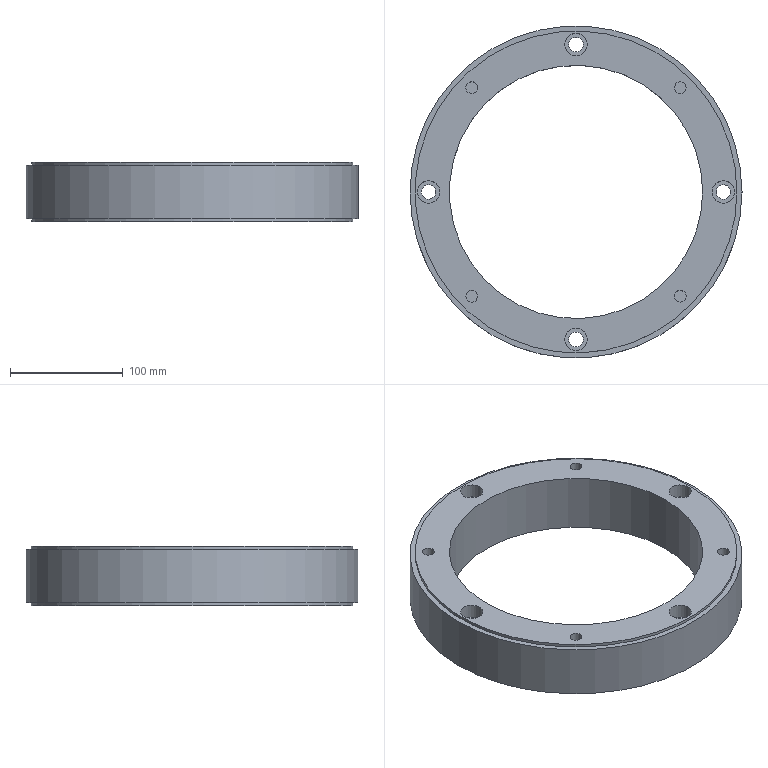Part | NX | 1 solid | 28 faces | box 295 x 295 x 53 mm | volume 1445870 mm3 | cylinder 16 | plane 12 | commonest cylinder face diameters 10.5 x4 13 x4 20 x4 286 x2 225 x1 295 x1
STEP:
#1=CARTESIAN_POINT('',(143.,0.,0.));
#2=VERTEX_POINT('',#1);
#3=CARTESIAN_POINT('',(0.,0.,0.));
#4=DIRECTION('',(0.,0.,1.));
#5=DIRECTION('',(1.,0.,0.));
#6=AXIS2_PLACEMENT_3D('',#3,#4,#5);
#7=CIRCLE('',#6,143.);
#8=EDGE_CURVE('',#2,#2,#7,.T.);
#9=ORIENTED_EDGE('',*,*,#8,.T.);
#10=EDGE_LOOP('',(#9));
#11=FACE_BOUND('',#10,.T.);
#12=CARTESIAN_POINT('',(112.5,0.,0.));
#13=VERTEX_POINT('',#12);
#14=CARTESIAN_POINT('',(0.,0.,0.));
#15=DIRECTION('',(0.,0.,1.));
#16=DIRECTION('',(1.,0.,0.));
#17=AXIS2_PLACEMENT_3D('',#14,#15,#16);
#18=CIRCLE('',#17,112.5);
#19=EDGE_CURVE('',#13,#13,#18,.T.);
#20=ORIENTED_EDGE('',*,*,#19,.F.);
#21=EDGE_LOOP('',(#20));
#22=FACE_BOUND('',#21,.T.);
#23=CARTESIAN_POINT('',(-131.,10.,0.));
#24=VERTEX_POINT('',#23);
#25=CARTESIAN_POINT('',(-131.,0.,0.));
#26=DIRECTION('',(0.,0.,1.));
#27=DIRECTION('',(0.,1.,0.));
#28=AXIS2_PLACEMENT_3D('',#25,#26,#27);
#29=CIRCLE('',#28,10.);
#30=EDGE_CURVE('',#24,#24,#29,.T.);
#31=ORIENTED_EDGE('',*,*,#30,.F.);
#32=EDGE_LOOP('',(#31));
#33=FACE_BOUND('',#32,.T.);
#34=CARTESIAN_POINT('',(-10.,-131.,0.));
#35=VERTEX_POINT('',#34);
#36=CARTESIAN_POINT('',(0.,-131.,0.));
#37=DIRECTION('',(0.,0.,1.));
#38=DIRECTION('',(-1.,0.,0.));
#39=AXIS2_PLACEMENT_3D('',#36,#37,#38);
#40=CIRCLE('',#39,10.);
#41=EDGE_CURVE('',#35,#35,#40,.T.);
#42=ORIENTED_EDGE('',*,*,#41,.F.);
#43=EDGE_LOOP('',(#42));
#44=FACE_BOUND('',#43,.T.);
#45=CARTESIAN_POINT('',(10.,131.,0.));
#46=VERTEX_POINT('',#45);
#47=CARTESIAN_POINT('',(0.,131.,0.));
#48=DIRECTION('',(0.,0.,1.));
#49=DIRECTION('',(1.,0.,0.));
#50=AXIS2_PLACEMENT_3D('',#47,#48,#49);
#51=CIRCLE('',#50,10.);
#52=EDGE_CURVE('',#46,#46,#51,.T.);
#53=ORIENTED_EDGE('',*,*,#52,.F.);
#54=EDGE_LOOP('',(#53));
#55=FACE_BOUND('',#54,.T.);
#56=CARTESIAN_POINT('',(131.,-10.,0.));
#57=VERTEX_POINT('',#56);
#58=CARTESIAN_POINT('',(131.,0.,0.));
#59=DIRECTION('',(0.,0.,1.));
#60=DIRECTION('',(0.,-1.,0.));
#61=AXIS2_PLACEMENT_3D('',#58,#59,#60);
#62=CIRCLE('',#61,10.);
#63=EDGE_CURVE('',#57,#57,#62,.T.);
#64=ORIENTED_EDGE('',*,*,#63,.F.);
#65=EDGE_LOOP('',(#64));
#66=FACE_BOUND('',#65,.T.);
#67=CARTESIAN_POINT('',(97.881,92.631,0.));
#68=VERTEX_POINT('',#67);
#69=CARTESIAN_POINT('',(92.631,92.631,0.));
#70=DIRECTION('',(0.,0.,1.));
#71=DIRECTION('',(1.,0.,0.));
#72=AXIS2_PLACEMENT_3D('',#69,#70,#71);
#73=CIRCLE('',#72,5.25);
#74=EDGE_CURVE('',#68,#68,#73,.T.);
#75=ORIENTED_EDGE('',*,*,#74,.F.);
#76=EDGE_LOOP('',(#75));
#77=FACE_BOUND('',#76,.T.);
#78=CARTESIAN_POINT('',(92.631,-97.881,0.));
#79=VERTEX_POINT('',#78);
#80=CARTESIAN_POINT('',(92.631,-92.631,0.));
#81=DIRECTION('',(0.,0.,1.));
#82=DIRECTION('',(0.,-1.,0.));
#83=AXIS2_PLACEMENT_3D('',#80,#81,#82);
#84=CIRCLE('',#83,5.25);
#85=EDGE_CURVE('',#79,#79,#84,.T.);
#86=ORIENTED_EDGE('',*,*,#85,.F.);
#87=EDGE_LOOP('',(#86));
#88=FACE_BOUND('',#87,.T.);
#89=CARTESIAN_POINT('',(-97.881,-92.631,0.));
#90=VERTEX_POINT('',#89);
#91=CARTESIAN_POINT('',(-92.631,-92.631,0.));
#92=DIRECTION('',(0.,0.,1.));
#93=DIRECTION('',(-1.,0.,0.));
#94=AXIS2_PLACEMENT_3D('',#91,#92,#93);
#95=CIRCLE('',#94,5.25);
#96=EDGE_CURVE('',#90,#90,#95,.T.);
#97=ORIENTED_EDGE('',*,*,#96,.F.);
#98=EDGE_LOOP('',(#97));
#99=FACE_BOUND('',#98,.T.);
#100=CARTESIAN_POINT('',(-92.631,97.881,0.));
#101=VERTEX_POINT('',#100);
#102=CARTESIAN_POINT('',(-92.631,92.631,0.));
#103=DIRECTION('',(0.,0.,-1.));
#104=DIRECTION('',(0.,1.,0.));
#105=AXIS2_PLACEMENT_3D('',#102,#103,#104);
#106=CIRCLE('',#105,5.25);
#107=EDGE_CURVE('',#101,#101,#106,.T.);
#108=ORIENTED_EDGE('',*,*,#107,.T.);
#109=EDGE_LOOP('',(#108));
#110=FACE_BOUND('',#109,.T.);
#111=CARTESIAN_POINT('',(65.5,0.,0.));
#112=DIRECTION('',(0.,0.,1.));
#113=DIRECTION('',(1.,0.,0.));
#114=AXIS2_PLACEMENT_3D('',#111,#112,#113);
#115=PLANE('',#114);
#116=ADVANCED_FACE('',(#11,#22,#33,#44,#55,#66,#77,#88,#99,#110),#115,.T.);
#117=CARTESIAN_POINT('',(-6.5,-131.,-53.));
#118=VERTEX_POINT('',#117);
#119=CARTESIAN_POINT('',(0.,-131.,-53.));
#120=DIRECTION('',(0.,0.,1.));
#121=DIRECTION('',(-1.,0.,0.));
#122=AXIS2_PLACEMENT_3D('',#119,#120,#121);
#123=CIRCLE('',#122,6.5);
#124=EDGE_CURVE('',#118,#118,#123,.T.);
#125=ORIENTED_EDGE('',*,*,#124,.F.);
#126=EDGE_LOOP('',(#125));
#127=FACE_BOUND('',#126,.T.);
#128=CARTESIAN_POINT('',(6.5,-131.,-13.));
#129=VERTEX_POINT('',#128);
#130=CARTESIAN_POINT('',(0.,-131.,-13.));
#131=DIRECTION('',(0.,0.,1.));
#132=DIRECTION('',(1.,0.,0.));
#133=AXIS2_PLACEMENT_3D('',#130,#131,#132);
#134=CIRCLE('',#133,6.5);
#135=EDGE_CURVE('',#129,#129,#134,.F.);
#136=ORIENTED_EDGE('',*,*,#135,.F.);
#137=EDGE_LOOP('',(#136));
#138=FACE_BOUND('',#137,.T.);
#139=CARTESIAN_POINT('',(0.,-131.,-53.));
#140=DIRECTION('',(0.,0.,1.));
#141=DIRECTION('',(1.,0.,0.));
#142=AXIS2_PLACEMENT_3D('',#139,#140,#141);
#143=CYLINDRICAL_SURFACE('',#142,6.5);
#144=ADVANCED_FACE('',(#127,#138),#143,.F.);
#145=CARTESIAN_POINT('',(6.5,131.,-53.));
#146=VERTEX_POINT('',#145);
#147=CARTESIAN_POINT('',(0.,131.,-53.));
#148=DIRECTION('',(0.,0.,1.));
#149=DIRECTION('',(1.,0.,0.));
#150=AXIS2_PLACEMENT_3D('',#147,#148,#149);
#151=CIRCLE('',#150,6.5);
#152=EDGE_CURVE('',#146,#146,#151,.T.);
#153=ORIENTED_EDGE('',*,*,#152,.F.);
#154=EDGE_LOOP('',(#153));
#155=FACE_BOUND('',#154,.T.);
#156=CARTESIAN_POINT('',(6.5,131.,-13.));
#157=VERTEX_POINT('',#156);
#158=CARTESIAN_POINT('',(0.,131.,-13.));
#159=DIRECTION('',(0.,0.,1.));
#160=DIRECTION('',(1.,0.,0.));
#161=AXIS2_PLACEMENT_3D('',#158,#159,#160);
#162=CIRCLE('',#161,6.5);
#163=EDGE_CURVE('',#157,#157,#162,.F.);
#164=ORIENTED_EDGE('',*,*,#163,.F.);
#165=EDGE_LOOP('',(#164));
#166=FACE_BOUND('',#165,.T.);
#167=CARTESIAN_POINT('',(0.,131.,-53.));
#168=DIRECTION('',(0.,0.,1.));
#169=DIRECTION('',(1.,0.,0.));
#170=AXIS2_PLACEMENT_3D('',#167,#168,#169);
#171=CYLINDRICAL_SURFACE('',#170,6.5);
#172=ADVANCED_FACE('',(#155,#166),#171,.F.);
#173=CARTESIAN_POINT('',(131.,-6.5,-53.));
#174=VERTEX_POINT('',#173);
#175=CARTESIAN_POINT('',(131.,0.,-53.));
#176=DIRECTION('',(0.,0.,1.));
#177=DIRECTION('',(0.,-1.,0.));
#178=AXIS2_PLACEMENT_3D('',#175,#176,#177);
#179=CIRCLE('',#178,6.5);
#180=EDGE_CURVE('',#174,#174,#179,.T.);
#181=ORIENTED_EDGE('',*,*,#180,.F.);
#182=EDGE_LOOP('',(#181));
#183=FACE_BOUND('',#182,.T.);
#184=CARTESIAN_POINT('',(137.5,0.,-13.));
#185=VERTEX_POINT('',#184);
#186=CARTESIAN_POINT('',(131.,0.,-13.));
#187=DIRECTION('',(0.,0.,1.));
#188=DIRECTION('',(1.,0.,0.));
#189=AXIS2_PLACEMENT_3D('',#186,#187,#188);
#190=CIRCLE('',#189,6.5);
#191=EDGE_CURVE('',#185,#185,#190,.F.);
#192=ORIENTED_EDGE('',*,*,#191,.F.);
#193=EDGE_LOOP('',(#192));
#194=FACE_BOUND('',#193,.T.);
#195=CARTESIAN_POINT('',(131.,0.,-53.));
#196=DIRECTION('',(0.,0.,1.));
#197=DIRECTION('',(1.,0.,0.));
#198=AXIS2_PLACEMENT_3D('',#195,#196,#197);
#199=CYLINDRICAL_SURFACE('',#198,6.5);
#200=ADVANCED_FACE('',(#183,#194),#199,.F.);
#201=CARTESIAN_POINT('',(-131.,6.5,-53.));
#202=VERTEX_POINT('',#201);
#203=CARTESIAN_POINT('',(-131.,0.,-53.));
#204=DIRECTION('',(0.,0.,1.));
#205=DIRECTION('',(0.,1.,0.));
#206=AXIS2_PLACEMENT_3D('',#203,#204,#205);
#207=CIRCLE('',#206,6.5);
#208=EDGE_CURVE('',#202,#202,#207,.T.);
#209=ORIENTED_EDGE('',*,*,#208,.F.);
#210=EDGE_LOOP('',(#209));
#211=FACE_BOUND('',#210,.T.);
#212=CARTESIAN_POINT('',(-124.5,0.,-13.));
#213=VERTEX_POINT('',#212);
#214=CARTESIAN_POINT('',(-131.,0.,-13.));
#215=DIRECTION('',(0.,0.,1.));
#216=DIRECTION('',(1.,0.,0.));
#217=AXIS2_PLACEMENT_3D('',#214,#215,#216);
#218=CIRCLE('',#217,6.5);
#219=EDGE_CURVE('',#213,#213,#218,.F.);
#220=ORIENTED_EDGE('',*,*,#219,.F.);
#221=EDGE_LOOP('',(#220));
#222=FACE_BOUND('',#221,.T.);
#223=CARTESIAN_POINT('',(-131.,0.,-53.));
#224=DIRECTION('',(0.,0.,1.));
#225=DIRECTION('',(1.,0.,0.));
#226=AXIS2_PLACEMENT_3D('',#223,#224,#225);
#227=CYLINDRICAL_SURFACE('',#226,6.5);
#228=ADVANCED_FACE('',(#211,#222),#227,.F.);
#229=CARTESIAN_POINT('',(147.5,0.,-2.6));
#230=VERTEX_POINT('',#229);
#231=CARTESIAN_POINT('',(0.,0.,-2.6));
#232=DIRECTION('',(0.,0.,-1.));
#233=DIRECTION('',(1.,0.,0.));
#234=AXIS2_PLACEMENT_3D('',#231,#232,#233);
#235=CIRCLE('',#234,147.5);
#236=EDGE_CURVE('',#230,#230,#235,.T.);
#237=ORIENTED_EDGE('',*,*,#236,.T.);
#238=EDGE_LOOP('',(#237));
#239=FACE_BOUND('',#238,.T.);
#240=CARTESIAN_POINT('',(147.5,0.,-50.4));
#241=VERTEX_POINT('',#240);
#242=CARTESIAN_POINT('',(0.,0.,-50.4));
#243=DIRECTION('',(0.,0.,-1.));
#244=DIRECTION('',(1.,0.,0.));
#245=AXIS2_PLACEMENT_3D('',#242,#243,#244);
#246=CIRCLE('',#245,147.5);
#247=EDGE_CURVE('',#241,#241,#246,.T.);
#248=ORIENTED_EDGE('',*,*,#247,.F.);
#249=EDGE_LOOP('',(#248));
#250=FACE_BOUND('',#249,.T.);
#251=CARTESIAN_POINT('',(0.,0.,-53.));
#252=DIRECTION('',(0.,0.,1.));
#253=DIRECTION('',(1.,0.,0.));
#254=AXIS2_PLACEMENT_3D('',#251,#252,#253);
#255=CYLINDRICAL_SURFACE('',#254,147.5);
#256=ADVANCED_FACE('',(#239,#250),#255,.T.);
#257=ORIENTED_EDGE('',*,*,#208,.T.);
#258=EDGE_LOOP('',(#257));
#259=FACE_BOUND('',#258,.T.);
#260=CARTESIAN_POINT('',(112.5,0.,-53.));
#261=VERTEX_POINT('',#260);
#262=CARTESIAN_POINT('',(0.,0.,-53.));
#263=DIRECTION('',(0.,0.,1.));
#264=DIRECTION('',(1.,0.,0.));
#265=AXIS2_PLACEMENT_3D('',#262,#263,#264);
#266=CIRCLE('',#265,112.5);
#267=EDGE_CURVE('',#261,#261,#266,.T.);
#268=ORIENTED_EDGE('',*,*,#267,.T.);
#269=EDGE_LOOP('',(#268));
#270=FACE_BOUND('',#269,.T.);
#271=ORIENTED_EDGE('',*,*,#124,.T.);
#272=EDGE_LOOP('',(#271));
#273=FACE_BOUND('',#272,.T.);
#274=ORIENTED_EDGE('',*,*,#152,.T.);
#275=EDGE_LOOP('',(#274));
#276=FACE_BOUND('',#275,.T.);
#277=ORIENTED_EDGE('',*,*,#180,.T.);
#278=EDGE_LOOP('',(#277));
#279=FACE_BOUND('',#278,.T.);
#280=CARTESIAN_POINT('',(143.,0.,-53.));
#281=VERTEX_POINT('',#280);
#282=CARTESIAN_POINT('',(0.,0.,-53.));
#283=DIRECTION('',(0.,0.,1.));
#284=DIRECTION('',(1.,0.,0.));
#285=AXIS2_PLACEMENT_3D('',#282,#283,#284);
#286=CIRCLE('',#285,143.);
#287=EDGE_CURVE('',#281,#281,#286,.T.);
#288=ORIENTED_EDGE('',*,*,#287,.F.);
#289=EDGE_LOOP('',(#288));
#290=FACE_BOUND('',#289,.T.);
#291=CARTESIAN_POINT('',(65.5,0.,-53.));
#292=DIRECTION('',(0.,0.,1.));
#293=DIRECTION('',(1.,0.,0.));
#294=AXIS2_PLACEMENT_3D('',#291,#292,#293);
#295=PLANE('',#294);
#296=ADVANCED_FACE('',(#259,#270,#273,#276,#279,#290),#295,.F.);
#297=ORIENTED_EDGE('',*,*,#267,.F.);
#298=EDGE_LOOP('',(#297));
#299=FACE_BOUND('',#298,.T.);
#300=ORIENTED_EDGE('',*,*,#19,.T.);
#301=EDGE_LOOP('',(#300));
#302=FACE_BOUND('',#301,.T.);
#303=CARTESIAN_POINT('',(0.,0.,-53.));
#304=DIRECTION('',(0.,0.,1.));
#305=DIRECTION('',(1.,0.,0.));
#306=AXIS2_PLACEMENT_3D('',#303,#304,#305);
#307=CYLINDRICAL_SURFACE('',#306,112.5);
#308=ADVANCED_FACE('',(#299,#302),#307,.F.);
#309=CARTESIAN_POINT('',(143.,0.,-2.6));
#310=VERTEX_POINT('',#309);
#311=CARTESIAN_POINT('',(0.,0.,-2.6));
#312=DIRECTION('',(0.,0.,1.));
#313=DIRECTION('',(1.,0.,0.));
#314=AXIS2_PLACEMENT_3D('',#311,#312,#313);
#315=CIRCLE('',#314,143.);
#316=EDGE_CURVE('',#310,#310,#315,.F.);
#317=ORIENTED_EDGE('',*,*,#316,.F.);
#318=EDGE_LOOP('',(#317));
#319=FACE_BOUND('',#318,.T.);
#320=ORIENTED_EDGE('',*,*,#8,.F.);
#321=EDGE_LOOP('',(#320));
#322=FACE_BOUND('',#321,.T.);
#323=CARTESIAN_POINT('',(0.,0.,-2.6));
#324=DIRECTION('',(0.,0.,1.));
#325=DIRECTION('',(1.,0.,0.));
#326=AXIS2_PLACEMENT_3D('',#323,#324,#325);
#327=CYLINDRICAL_SURFACE('',#326,143.);
#328=ADVANCED_FACE('',(#319,#322),#327,.T.);
#329=ORIENTED_EDGE('',*,*,#236,.F.);
#330=EDGE_LOOP('',(#329));
#331=FACE_BOUND('',#330,.T.);
#332=ORIENTED_EDGE('',*,*,#316,.T.);
#333=EDGE_LOOP('',(#332));
#334=FACE_BOUND('',#333,.T.);
#335=CARTESIAN_POINT('',(0.,0.,-2.6));
#336=DIRECTION('',(0.,0.,-1.));
#337=DIRECTION('',(-1.,0.,0.));
#338=AXIS2_PLACEMENT_3D('',#335,#336,#337);
#339=PLANE('',#338);
#340=ADVANCED_FACE('',(#331,#334),#339,.F.);
#341=CARTESIAN_POINT('',(143.,0.,-50.4));
#342=VERTEX_POINT('',#341);
#343=CARTESIAN_POINT('',(0.,0.,-50.4));
#344=DIRECTION('',(0.,0.,1.));
#345=DIRECTION('',(1.,0.,0.));
#346=AXIS2_PLACEMENT_3D('',#343,#344,#345);
#347=CIRCLE('',#346,143.);
#348=EDGE_CURVE('',#342,#342,#347,.F.);
#349=ORIENTED_EDGE('',*,*,#348,.T.);
#350=EDGE_LOOP('',(#349));
#351=FACE_BOUND('',#350,.T.);
#352=ORIENTED_EDGE('',*,*,#287,.T.);
#353=EDGE_LOOP('',(#352));
#354=FACE_BOUND('',#353,.T.);
#355=CARTESIAN_POINT('',(0.,0.,-50.4));
#356=DIRECTION('',(0.,0.,-1.));
#357=DIRECTION('',(-1.,0.,0.));
#358=AXIS2_PLACEMENT_3D('',#355,#356,#357);
#359=CYLINDRICAL_SURFACE('',#358,143.);
#360=ADVANCED_FACE('',(#351,#354),#359,.T.);
#361=ORIENTED_EDGE('',*,*,#247,.T.);
#362=EDGE_LOOP('',(#361));
#363=FACE_BOUND('',#362,.T.);
#364=ORIENTED_EDGE('',*,*,#348,.F.);
#365=EDGE_LOOP('',(#364));
#366=FACE_BOUND('',#365,.T.);
#367=CARTESIAN_POINT('',(0.,0.,-50.4));
#368=DIRECTION('',(0.,0.,-1.));
#369=DIRECTION('',(-1.,0.,0.));
#370=AXIS2_PLACEMENT_3D('',#367,#368,#369);
#371=PLANE('',#370);
#372=ADVANCED_FACE('',(#363,#366),#371,.T.);
#373=CARTESIAN_POINT('',(-131.,10.,-13.));
#374=VERTEX_POINT('',#373);
#375=CARTESIAN_POINT('',(-131.,0.,-13.));
#376=DIRECTION('',(0.,0.,1.));
#377=DIRECTION('',(0.,1.,0.));
#378=AXIS2_PLACEMENT_3D('',#375,#376,#377);
#379=CIRCLE('',#378,10.);
#380=EDGE_CURVE('',#374,#374,#379,.F.);
#381=ORIENTED_EDGE('',*,*,#380,.F.);
#382=EDGE_LOOP('',(#381));
#383=FACE_BOUND('',#382,.T.);
#384=ORIENTED_EDGE('',*,*,#219,.T.);
#385=EDGE_LOOP('',(#384));
#386=FACE_BOUND('',#385,.T.);
#387=CARTESIAN_POINT('',(-131.,0.,-13.));
#388=DIRECTION('',(0.,0.,1.));
#389=DIRECTION('',(1.,0.,0.));
#390=AXIS2_PLACEMENT_3D('',#387,#388,#389);
#391=PLANE('',#390);
#392=ADVANCED_FACE('',(#383,#386),#391,.T.);
#393=ORIENTED_EDGE('',*,*,#380,.T.);
#394=EDGE_LOOP('',(#393));
#395=FACE_BOUND('',#394,.T.);
#396=ORIENTED_EDGE('',*,*,#30,.T.);
#397=EDGE_LOOP('',(#396));
#398=FACE_BOUND('',#397,.T.);
#399=CARTESIAN_POINT('',(-131.,0.,-13.));
#400=DIRECTION('',(0.,0.,1.));
#401=DIRECTION('',(1.,0.,0.));
#402=AXIS2_PLACEMENT_3D('',#399,#400,#401);
#403=CYLINDRICAL_SURFACE('',#402,10.);
#404=ADVANCED_FACE('',(#395,#398),#403,.F.);
#405=CARTESIAN_POINT('',(131.,-10.,-13.));
#406=VERTEX_POINT('',#405);
#407=CARTESIAN_POINT('',(131.,0.,-13.));
#408=DIRECTION('',(0.,0.,1.));
#409=DIRECTION('',(0.,-1.,0.));
#410=AXIS2_PLACEMENT_3D('',#407,#408,#409);
#411=CIRCLE('',#410,10.);
#412=EDGE_CURVE('',#406,#406,#411,.F.);
#413=ORIENTED_EDGE('',*,*,#412,.F.);
#414=EDGE_LOOP('',(#413));
#415=FACE_BOUND('',#414,.T.);
#416=ORIENTED_EDGE('',*,*,#191,.T.);
#417=EDGE_LOOP('',(#416));
#418=FACE_BOUND('',#417,.T.);
#419=CARTESIAN_POINT('',(131.,0.,-13.));
#420=DIRECTION('',(0.,0.,1.));
#421=DIRECTION('',(1.,0.,0.));
#422=AXIS2_PLACEMENT_3D('',#419,#420,#421);
#423=PLANE('',#422);
#424=ADVANCED_FACE('',(#415,#418),#423,.T.);
#425=ORIENTED_EDGE('',*,*,#412,.T.);
#426=EDGE_LOOP('',(#425));
#427=FACE_BOUND('',#426,.T.);
#428=ORIENTED_EDGE('',*,*,#63,.T.);
#429=EDGE_LOOP('',(#428));
#430=FACE_BOUND('',#429,.T.);
#431=CARTESIAN_POINT('',(131.,0.,-13.));
#432=DIRECTION('',(0.,0.,1.));
#433=DIRECTION('',(1.,0.,0.));
#434=AXIS2_PLACEMENT_3D('',#431,#432,#433);
#435=CYLINDRICAL_SURFACE('',#434,10.);
#436=ADVANCED_FACE('',(#427,#430),#435,.F.);
#437=CARTESIAN_POINT('',(10.,131.,-13.));
#438=VERTEX_POINT('',#437);
#439=CARTESIAN_POINT('',(0.,131.,-13.));
#440=DIRECTION('',(0.,0.,1.));
#441=DIRECTION('',(1.,0.,0.));
#442=AXIS2_PLACEMENT_3D('',#439,#440,#441);
#443=CIRCLE('',#442,10.);
#444=EDGE_CURVE('',#438,#438,#443,.F.);
#445=ORIENTED_EDGE('',*,*,#444,.F.);
#446=EDGE_LOOP('',(#445));
#447=FACE_BOUND('',#446,.T.);
#448=ORIENTED_EDGE('',*,*,#163,.T.);
#449=EDGE_LOOP('',(#448));
#450=FACE_BOUND('',#449,.T.);
#451=CARTESIAN_POINT('',(0.,131.,-13.));
#452=DIRECTION('',(0.,0.,1.));
#453=DIRECTION('',(1.,0.,0.));
#454=AXIS2_PLACEMENT_3D('',#451,#452,#453);
#455=PLANE('',#454);
#456=ADVANCED_FACE('',(#447,#450),#455,.T.);
#457=ORIENTED_EDGE('',*,*,#444,.T.);
#458=EDGE_LOOP('',(#457));
#459=FACE_BOUND('',#458,.T.);
#460=ORIENTED_EDGE('',*,*,#52,.T.);
#461=EDGE_LOOP('',(#460));
#462=FACE_BOUND('',#461,.T.);
#463=CARTESIAN_POINT('',(0.,131.,-13.));
#464=DIRECTION('',(0.,0.,1.));
#465=DIRECTION('',(1.,0.,0.));
#466=AXIS2_PLACEMENT_3D('',#463,#464,#465);
#467=CYLINDRICAL_SURFACE('',#466,10.);
#468=ADVANCED_FACE('',(#459,#462),#467,.F.);
#469=CARTESIAN_POINT('',(-10.,-131.,-13.));
#470=VERTEX_POINT('',#469);
#471=CARTESIAN_POINT('',(0.,-131.,-13.));
#472=DIRECTION('',(0.,0.,1.));
#473=DIRECTION('',(-1.,0.,0.));
#474=AXIS2_PLACEMENT_3D('',#471,#472,#473);
#475=CIRCLE('',#474,10.);
#476=EDGE_CURVE('',#470,#470,#475,.F.);
#477=ORIENTED_EDGE('',*,*,#476,.F.);
#478=EDGE_LOOP('',(#477));
#479=FACE_BOUND('',#478,.T.);
#480=ORIENTED_EDGE('',*,*,#135,.T.);
#481=EDGE_LOOP('',(#480));
#482=FACE_BOUND('',#481,.T.);
#483=CARTESIAN_POINT('',(0.,-131.,-13.));
#484=DIRECTION('',(0.,0.,1.));
#485=DIRECTION('',(1.,0.,0.));
#486=AXIS2_PLACEMENT_3D('',#483,#484,#485);
#487=PLANE('',#486);
#488=ADVANCED_FACE('',(#479,#482),#487,.T.);
#489=ORIENTED_EDGE('',*,*,#476,.T.);
#490=EDGE_LOOP('',(#489));
#491=FACE_BOUND('',#490,.T.);
#492=ORIENTED_EDGE('',*,*,#41,.T.);
#493=EDGE_LOOP('',(#492));
#494=FACE_BOUND('',#493,.T.);
#495=CARTESIAN_POINT('',(0.,-131.,-13.));
#496=DIRECTION('',(0.,0.,1.));
#497=DIRECTION('',(1.,0.,0.));
#498=AXIS2_PLACEMENT_3D('',#495,#496,#497);
#499=CYLINDRICAL_SURFACE('',#498,10.);
#500=ADVANCED_FACE('',(#491,#494),#499,.F.);
#501=CARTESIAN_POINT('',(97.881,92.631,-30.));
#502=VERTEX_POINT('',#501);
#503=CARTESIAN_POINT('',(92.631,92.631,-30.));
#504=DIRECTION('',(0.,0.,1.));
#505=DIRECTION('',(1.,0.,0.));
#506=AXIS2_PLACEMENT_3D('',#503,#504,#505);
#507=CIRCLE('',#506,5.25);
#508=EDGE_CURVE('',#502,#502,#507,.F.);
#509=ORIENTED_EDGE('',*,*,#508,.T.);
#510=EDGE_LOOP('',(#509));
#511=FACE_BOUND('',#510,.T.);
#512=ORIENTED_EDGE('',*,*,#74,.T.);
#513=EDGE_LOOP('',(#512));
#514=FACE_BOUND('',#513,.T.);
#515=CARTESIAN_POINT('',(92.631,92.631,-30.));
#516=DIRECTION('',(0.,0.,1.));
#517=DIRECTION('',(1.,0.,0.));
#518=AXIS2_PLACEMENT_3D('',#515,#516,#517);
#519=CYLINDRICAL_SURFACE('',#518,5.25);
#520=ADVANCED_FACE('',(#511,#514),#519,.F.);
#521=ORIENTED_EDGE('',*,*,#508,.F.);
#522=EDGE_LOOP('',(#521));
#523=FACE_BOUND('',#522,.T.);
#524=CARTESIAN_POINT('',(92.631,92.631,-30.));
#525=DIRECTION('',(0.,0.,1.));
#526=DIRECTION('',(1.,0.,0.));
#527=AXIS2_PLACEMENT_3D('',#524,#525,#526);
#528=PLANE('',#527);
#529=ADVANCED_FACE('',(#523),#528,.T.);
#530=CARTESIAN_POINT('',(92.631,-97.881,-30.));
#531=VERTEX_POINT('',#530);
#532=CARTESIAN_POINT('',(92.631,-92.631,-30.));
#533=DIRECTION('',(0.,0.,1.));
#534=DIRECTION('',(0.,-1.,0.));
#535=AXIS2_PLACEMENT_3D('',#532,#533,#534);
#536=CIRCLE('',#535,5.25);
#537=EDGE_CURVE('',#531,#531,#536,.F.);
#538=ORIENTED_EDGE('',*,*,#537,.T.);
#539=EDGE_LOOP('',(#538));
#540=FACE_BOUND('',#539,.T.);
#541=ORIENTED_EDGE('',*,*,#85,.T.);
#542=EDGE_LOOP('',(#541));
#543=FACE_BOUND('',#542,.T.);
#544=CARTESIAN_POINT('',(92.631,-92.631,-30.));
#545=DIRECTION('',(0.,0.,1.));
#546=DIRECTION('',(1.,0.,0.));
#547=AXIS2_PLACEMENT_3D('',#544,#545,#546);
#548=CYLINDRICAL_SURFACE('',#547,5.25);
#549=ADVANCED_FACE('',(#540,#543),#548,.F.);
#550=ORIENTED_EDGE('',*,*,#537,.F.);
#551=EDGE_LOOP('',(#550));
#552=FACE_BOUND('',#551,.T.);
#553=CARTESIAN_POINT('',(92.631,-92.631,-30.));
#554=DIRECTION('',(0.,0.,1.));
#555=DIRECTION('',(1.,0.,0.));
#556=AXIS2_PLACEMENT_3D('',#553,#554,#555);
#557=PLANE('',#556);
#558=ADVANCED_FACE('',(#552),#557,.T.);
#559=CARTESIAN_POINT('',(-97.881,-92.631,-30.));
#560=VERTEX_POINT('',#559);
#561=CARTESIAN_POINT('',(-92.631,-92.631,-30.));
#562=DIRECTION('',(0.,0.,1.));
#563=DIRECTION('',(-1.,0.,0.));
#564=AXIS2_PLACEMENT_3D('',#561,#562,#563);
#565=CIRCLE('',#564,5.25);
#566=EDGE_CURVE('',#560,#560,#565,.F.);
#567=ORIENTED_EDGE('',*,*,#566,.T.);
#568=EDGE_LOOP('',(#567));
#569=FACE_BOUND('',#568,.T.);
#570=ORIENTED_EDGE('',*,*,#96,.T.);
#571=EDGE_LOOP('',(#570));
#572=FACE_BOUND('',#571,.T.);
#573=CARTESIAN_POINT('',(-92.631,-92.631,-30.));
#574=DIRECTION('',(0.,0.,1.));
#575=DIRECTION('',(1.,0.,0.));
#576=AXIS2_PLACEMENT_3D('',#573,#574,#575);
#577=CYLINDRICAL_SURFACE('',#576,5.25);
#578=ADVANCED_FACE('',(#569,#572),#577,.F.);
#579=ORIENTED_EDGE('',*,*,#566,.F.);
#580=EDGE_LOOP('',(#579));
#581=FACE_BOUND('',#580,.T.);
#582=CARTESIAN_POINT('',(-92.631,-92.631,-30.));
#583=DIRECTION('',(0.,0.,1.));
#584=DIRECTION('',(1.,0.,0.));
#585=AXIS2_PLACEMENT_3D('',#582,#583,#584);
#586=PLANE('',#585);
#587=ADVANCED_FACE('',(#581),#586,.T.);
#588=CARTESIAN_POINT('',(-92.631,97.881,-30.));
#589=VERTEX_POINT('',#588);
#590=CARTESIAN_POINT('',(-92.631,92.631,-30.));
#591=DIRECTION('',(0.,0.,-1.));
#592=DIRECTION('',(0.,1.,0.));
#593=AXIS2_PLACEMENT_3D('',#590,#591,#592);
#594=CIRCLE('',#593,5.25);
#595=EDGE_CURVE('',#589,#589,#594,.F.);
#596=ORIENTED_EDGE('',*,*,#595,.F.);
#597=EDGE_LOOP('',(#596));
#598=FACE_BOUND('',#597,.T.);
#599=ORIENTED_EDGE('',*,*,#107,.F.);
#600=EDGE_LOOP('',(#599));
#601=FACE_BOUND('',#600,.T.);
#602=CARTESIAN_POINT('',(-92.631,92.631,-30.));
#603=DIRECTION('',(0.,0.,1.));
#604=DIRECTION('',(1.,0.,0.));
#605=AXIS2_PLACEMENT_3D('',#602,#603,#604);
#606=CYLINDRICAL_SURFACE('',#605,5.25);
#607=ADVANCED_FACE('',(#598,#601),#606,.F.);
#608=ORIENTED_EDGE('',*,*,#595,.T.);
#609=EDGE_LOOP('',(#608));
#610=FACE_BOUND('',#609,.T.);
#611=CARTESIAN_POINT('',(-92.631,92.631,-30.));
#612=DIRECTION('',(0.,0.,-1.));
#613=DIRECTION('',(-1.,0.,0.));
#614=AXIS2_PLACEMENT_3D('',#611,#612,#613);
#615=PLANE('',#614);
#616=ADVANCED_FACE('',(#610),#615,.F.);
#617=CLOSED_SHELL('',(#116,#144,#172,#200,#228,#256,#296,#308,#328,#340,#360,#372,#392,#404,#424,#436,#456,#468,#488,#500,#520,#529,#549,#558,#578,#587,#607,#616));
#618=MANIFOLD_SOLID_BREP('',#617);
#619=(LENGTH_UNIT()NAMED_UNIT(*)SI_UNIT(.MILLI.,.METRE.));
#620=UNCERTAINTY_MEASURE_WITH_UNIT(LENGTH_MEASURE(0.00001),#619,'','');
#621=(NAMED_UNIT(*)PLANE_ANGLE_UNIT()SI_UNIT($,.RADIAN.));
#622=(NAMED_UNIT(*)SI_UNIT($,.STERADIAN.)SOLID_ANGLE_UNIT());
#623=(GEOMETRIC_REPRESENTATION_CONTEXT(3)GLOBAL_UNCERTAINTY_ASSIGNED_CONTEXT((#620))GLOBAL_UNIT_ASSIGNED_CONTEXT((#619,#621,#622))REPRESENTATION_CONTEXT('',''));
#624=ADVANCED_BREP_SHAPE_REPRESENTATION('',(#618),#623);